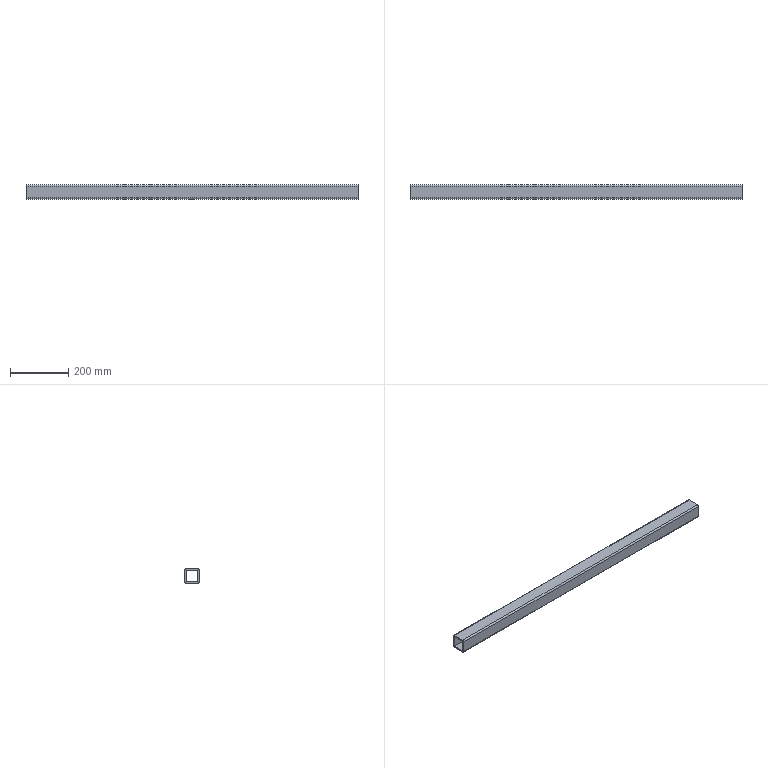Part | STEP file | SOLID | 1 solid | 15 faces | box 1140 x 50 x 50 mm | volume 1000530 mm3 | plane 10 | cylinder 5 | commonest cylinder face diameters 10 x4 16 x1
STEP:
#1=CARTESIAN_POINT('',(0.,0.,0.));
#2=DIRECTION('',(0.,0.,1.));
#3=DIRECTION('',(1.,0.,0.));
#4=AXIS2_PLACEMENT_3D('',#1,#2,#3);
#5=CARTESIAN_POINT('',(-753.5,420.,-725.));
#6=VERTEX_POINT('',#5);
#7=CARTESIAN_POINT('',(-753.5,420.,-685.));
#8=VERTEX_POINT('',#7);
#9=CARTESIAN_POINT('',(-753.5,420.,-685.));
#10=DIRECTION('',(0.,0.,1.));
#11=VECTOR('',#10,1.);
#12=LINE('',#9,#11);
#13=CARTESIAN_POINT('',(636.5,420.,-685.));
#14=DIRECTION('',(0.,-1.,0.));
#15=DIRECTION('',(0.,0.,1.));
#16=AXIS2_PLACEMENT_3D('',#13,#14,#15);
#17=PLANE('',#16);
#18=CARTESIAN_POINT('',(0.,1390.));
#19=DIRECTION('',(1.,0.));
#20=VECTOR('',#19,1.);
#21=LINE('',#18,#20);
#22=(GEOMETRIC_REPRESENTATION_CONTEXT(2)PARAMETRIC_REPRESENTATION_CONTEXT()REPRESENTATION_CONTEXT('',''));
#23=DEFINITIONAL_REPRESENTATION('',(#21),#22);
#24=PCURVE('',#17,#23);
#25=CARTESIAN_POINT('',(-753.5,380.,-670.));
#26=DIRECTION('',(-1.,0.,0.));
#27=DIRECTION('',(0.,1.,0.));
#28=AXIS2_PLACEMENT_3D('',#25,#26,#27);
#29=PLANE('',#28);
#30=CARTESIAN_POINT('',(40.,15.));
#31=DIRECTION('',(0.,-1.));
#32=VECTOR('',#31,1.);
#33=LINE('',#30,#32);
#34=(GEOMETRIC_REPRESENTATION_CONTEXT(2)PARAMETRIC_REPRESENTATION_CONTEXT()REPRESENTATION_CONTEXT('',''));
#35=DEFINITIONAL_REPRESENTATION('',(#33),#34);
#36=PCURVE('',#29,#35);
#37=SURFACE_CURVE('',#12,(#24,#36),.PCURVE_S1.);
#38=EDGE_CURVE('',#6,#8,#37,.T.);
#39=ORIENTED_EDGE('',*,*,#38,.F.);
#40=CARTESIAN_POINT('',(386.5,420.,-725.));
#41=VERTEX_POINT('',#40);
#42=CARTESIAN_POINT('',(636.5,420.,-725.));
#43=DIRECTION('',(1.,0.,0.));
#44=VECTOR('',#43,1.);
#45=LINE('',#42,#44);
#46=CARTESIAN_POINT('',(-40.,0.));
#47=DIRECTION('',(0.,-1.));
#48=VECTOR('',#47,1.);
#49=LINE('',#46,#48);
#50=(GEOMETRIC_REPRESENTATION_CONTEXT(2)PARAMETRIC_REPRESENTATION_CONTEXT()REPRESENTATION_CONTEXT('',''));
#51=DEFINITIONAL_REPRESENTATION('',(#49),#50);
#52=PCURVE('',#17,#51);
#53=CARTESIAN_POINT('',(636.5,420.,-725.));
#54=DIRECTION('',(0.,0.,1.));
#55=DIRECTION('',(0.,1.,0.));
#56=AXIS2_PLACEMENT_3D('',#53,#54,#55);
#57=PLANE('',#56);
#58=CARTESIAN_POINT('',(0.,0.));
#59=DIRECTION('',(0.,-1.));
#60=VECTOR('',#59,1.);
#61=LINE('',#58,#60);
#62=(GEOMETRIC_REPRESENTATION_CONTEXT(2)PARAMETRIC_REPRESENTATION_CONTEXT()REPRESENTATION_CONTEXT('',''));
#63=DEFINITIONAL_REPRESENTATION('',(#61),#62);
#64=PCURVE('',#57,#63);
#65=SURFACE_CURVE('',#45,(#52,#64),.PCURVE_S1.);
#66=EDGE_CURVE('',#6,#41,#65,.T.);
#67=ORIENTED_EDGE('',*,*,#66,.T.);
#68=CARTESIAN_POINT('',(386.5,420.,-685.));
#69=VERTEX_POINT('',#68);
#70=CARTESIAN_POINT('',(386.5,420.,-685.));
#71=DIRECTION('',(0.,0.,1.));
#72=VECTOR('',#71,1.);
#73=LINE('',#70,#72);
#74=CARTESIAN_POINT('',(0.,250.));
#75=DIRECTION('',(1.,0.));
#76=VECTOR('',#75,1.);
#77=LINE('',#74,#76);
#78=(GEOMETRIC_REPRESENTATION_CONTEXT(2)PARAMETRIC_REPRESENTATION_CONTEXT()REPRESENTATION_CONTEXT('',''));
#79=DEFINITIONAL_REPRESENTATION('',(#77),#78);
#80=PCURVE('',#17,#79);
#81=CARTESIAN_POINT('',(386.5,380.,-670.));
#82=DIRECTION('',(1.,0.,0.));
#83=DIRECTION('',(0.,1.,0.));
#84=AXIS2_PLACEMENT_3D('',#81,#82,#83);
#85=PLANE('',#84);
#86=CARTESIAN_POINT('',(40.,-15.));
#87=DIRECTION('',(0.,1.));
#88=VECTOR('',#87,1.);
#89=LINE('',#86,#88);
#90=(GEOMETRIC_REPRESENTATION_CONTEXT(2)PARAMETRIC_REPRESENTATION_CONTEXT()REPRESENTATION_CONTEXT('',''));
#91=DEFINITIONAL_REPRESENTATION('',(#89),#90);
#92=PCURVE('',#85,#91);
#93=SURFACE_CURVE('',#73,(#80,#92),.PCURVE_S1.);
#94=EDGE_CURVE('',#41,#69,#93,.T.);
#95=ORIENTED_EDGE('',*,*,#94,.T.);
#96=CARTESIAN_POINT('',(636.5,420.,-685.));
#97=DIRECTION('',(1.,0.,0.));
#98=VECTOR('',#97,1.);
#99=LINE('',#96,#98);
#100=CARTESIAN_POINT('',(0.,0.));
#101=DIRECTION('',(0.,-1.));
#102=VECTOR('',#101,1.);
#103=LINE('',#100,#102);
#104=(GEOMETRIC_REPRESENTATION_CONTEXT(2)PARAMETRIC_REPRESENTATION_CONTEXT()REPRESENTATION_CONTEXT('',''));
#105=DEFINITIONAL_REPRESENTATION('',(#103),#104);
#106=PCURVE('',#17,#105);
#107=CARTESIAN_POINT('',(636.5,380.,-685.));
#108=DIRECTION('',(0.,0.,-1.));
#109=DIRECTION('',(0.,-1.,0.));
#110=AXIS2_PLACEMENT_3D('',#107,#108,#109);
#111=PLANE('',#110);
#112=CARTESIAN_POINT('',(-40.,0.));
#113=DIRECTION('',(0.,-1.));
#114=VECTOR('',#113,1.);
#115=LINE('',#112,#114);
#116=(GEOMETRIC_REPRESENTATION_CONTEXT(2)PARAMETRIC_REPRESENTATION_CONTEXT()REPRESENTATION_CONTEXT('',''));
#117=DEFINITIONAL_REPRESENTATION('',(#115),#116);
#118=PCURVE('',#111,#117);
#119=SURFACE_CURVE('',#99,(#106,#118),.PCURVE_S1.);
#120=EDGE_CURVE('',#8,#69,#119,.T.);
#121=ORIENTED_EDGE('',*,*,#120,.F.);
#122=EDGE_LOOP('',(#39,#67,#95,#121));
#123=FACE_BOUND('',#122,.T.);
#124=ADVANCED_FACE('',(#123),#17,.T.);
#125=CARTESIAN_POINT('',(-753.5,380.,-685.));
#126=VERTEX_POINT('',#125);
#127=CARTESIAN_POINT('',(-753.5,380.,-685.));
#128=DIRECTION('',(0.,-1.,0.));
#129=VECTOR('',#128,1.);
#130=LINE('',#127,#129);
#131=CARTESIAN_POINT('',(0.,1390.));
#132=DIRECTION('',(1.,0.));
#133=VECTOR('',#132,1.);
#134=LINE('',#131,#133);
#135=(GEOMETRIC_REPRESENTATION_CONTEXT(2)PARAMETRIC_REPRESENTATION_CONTEXT()REPRESENTATION_CONTEXT('',''));
#136=DEFINITIONAL_REPRESENTATION('',(#134),#135);
#137=PCURVE('',#111,#136);
#138=CARTESIAN_POINT('',(0.,15.));
#139=DIRECTION('',(-1.,0.));
#140=VECTOR('',#139,1.);
#141=LINE('',#138,#140);
#142=(GEOMETRIC_REPRESENTATION_CONTEXT(2)PARAMETRIC_REPRESENTATION_CONTEXT()REPRESENTATION_CONTEXT('',''));
#143=DEFINITIONAL_REPRESENTATION('',(#141),#142);
#144=PCURVE('',#29,#143);
#145=SURFACE_CURVE('',#130,(#137,#144),.PCURVE_S1.);
#146=EDGE_CURVE('',#8,#126,#145,.T.);
#147=ORIENTED_EDGE('',*,*,#146,.F.);
#148=ORIENTED_EDGE('',*,*,#120,.T.);
#149=CARTESIAN_POINT('',(386.5,380.,-685.));
#150=VERTEX_POINT('',#149);
#151=CARTESIAN_POINT('',(386.5,380.,-685.));
#152=DIRECTION('',(0.,-1.,0.));
#153=VECTOR('',#152,1.);
#154=LINE('',#151,#153);
#155=CARTESIAN_POINT('',(0.,250.));
#156=DIRECTION('',(1.,0.));
#157=VECTOR('',#156,1.);
#158=LINE('',#155,#157);
#159=(GEOMETRIC_REPRESENTATION_CONTEXT(2)PARAMETRIC_REPRESENTATION_CONTEXT()REPRESENTATION_CONTEXT('',''));
#160=DEFINITIONAL_REPRESENTATION('',(#158),#159);
#161=PCURVE('',#111,#160);
#162=CARTESIAN_POINT('',(0.,-15.));
#163=DIRECTION('',(-1.,0.));
#164=VECTOR('',#163,1.);
#165=LINE('',#162,#164);
#166=(GEOMETRIC_REPRESENTATION_CONTEXT(2)PARAMETRIC_REPRESENTATION_CONTEXT()REPRESENTATION_CONTEXT('',''));
#167=DEFINITIONAL_REPRESENTATION('',(#165),#166);
#168=PCURVE('',#85,#167);
#169=SURFACE_CURVE('',#154,(#161,#168),.PCURVE_S1.);
#170=EDGE_CURVE('',#69,#150,#169,.T.);
#171=ORIENTED_EDGE('',*,*,#170,.T.);
#172=CARTESIAN_POINT('',(636.5,380.,-685.));
#173=DIRECTION('',(1.,0.,0.));
#174=VECTOR('',#173,1.);
#175=LINE('',#172,#174);
#176=CARTESIAN_POINT('',(0.,0.));
#177=DIRECTION('',(0.,-1.));
#178=VECTOR('',#177,1.);
#179=LINE('',#176,#178);
#180=(GEOMETRIC_REPRESENTATION_CONTEXT(2)PARAMETRIC_REPRESENTATION_CONTEXT()REPRESENTATION_CONTEXT('',''));
#181=DEFINITIONAL_REPRESENTATION('',(#179),#180);
#182=PCURVE('',#111,#181);
#183=CARTESIAN_POINT('',(636.5,380.,-725.));
#184=DIRECTION('',(0.,1.,0.));
#185=DIRECTION('',(0.,0.,-1.));
#186=AXIS2_PLACEMENT_3D('',#183,#184,#185);
#187=PLANE('',#186);
#188=CARTESIAN_POINT('',(-40.,0.));
#189=DIRECTION('',(0.,-1.));
#190=VECTOR('',#189,1.);
#191=LINE('',#188,#190);
#192=(GEOMETRIC_REPRESENTATION_CONTEXT(2)PARAMETRIC_REPRESENTATION_CONTEXT()REPRESENTATION_CONTEXT('',''));
#193=DEFINITIONAL_REPRESENTATION('',(#191),#192);
#194=PCURVE('',#187,#193);
#195=SURFACE_CURVE('',#175,(#182,#194),.PCURVE_S1.);
#196=EDGE_CURVE('',#126,#150,#195,.T.);
#197=ORIENTED_EDGE('',*,*,#196,.F.);
#198=EDGE_LOOP('',(#147,#148,#171,#197));
#199=FACE_BOUND('',#198,.T.);
#200=ADVANCED_FACE('',(#199),#111,.T.);
#201=CARTESIAN_POINT('',(-753.5,380.,-725.));
#202=VERTEX_POINT('',#201);
#203=CARTESIAN_POINT('',(-753.5,380.,-725.));
#204=DIRECTION('',(0.,0.,-1.));
#205=VECTOR('',#204,1.);
#206=LINE('',#203,#205);
#207=CARTESIAN_POINT('',(0.,1390.));
#208=DIRECTION('',(1.,0.));
#209=VECTOR('',#208,1.);
#210=LINE('',#207,#209);
#211=(GEOMETRIC_REPRESENTATION_CONTEXT(2)PARAMETRIC_REPRESENTATION_CONTEXT()REPRESENTATION_CONTEXT('',''));
#212=DEFINITIONAL_REPRESENTATION('',(#210),#211);
#213=PCURVE('',#187,#212);
#214=CARTESIAN_POINT('',(0.,55.));
#215=DIRECTION('',(0.,1.));
#216=VECTOR('',#215,1.);
#217=LINE('',#214,#216);
#218=(GEOMETRIC_REPRESENTATION_CONTEXT(2)PARAMETRIC_REPRESENTATION_CONTEXT()REPRESENTATION_CONTEXT('',''));
#219=DEFINITIONAL_REPRESENTATION('',(#217),#218);
#220=PCURVE('',#29,#219);
#221=SURFACE_CURVE('',#206,(#213,#220),.PCURVE_S1.);
#222=EDGE_CURVE('',#126,#202,#221,.T.);
#223=ORIENTED_EDGE('',*,*,#222,.F.);
#224=ORIENTED_EDGE('',*,*,#196,.T.);
#225=CARTESIAN_POINT('',(386.5,380.,-725.));
#226=VERTEX_POINT('',#225);
#227=CARTESIAN_POINT('',(386.5,380.,-725.));
#228=DIRECTION('',(0.,0.,-1.));
#229=VECTOR('',#228,1.);
#230=LINE('',#227,#229);
#231=CARTESIAN_POINT('',(0.,250.));
#232=DIRECTION('',(1.,0.));
#233=VECTOR('',#232,1.);
#234=LINE('',#231,#233);
#235=(GEOMETRIC_REPRESENTATION_CONTEXT(2)PARAMETRIC_REPRESENTATION_CONTEXT()REPRESENTATION_CONTEXT('',''));
#236=DEFINITIONAL_REPRESENTATION('',(#234),#235);
#237=PCURVE('',#187,#236);
#238=CARTESIAN_POINT('',(0.,-55.));
#239=DIRECTION('',(0.,-1.));
#240=VECTOR('',#239,1.);
#241=LINE('',#238,#240);
#242=(GEOMETRIC_REPRESENTATION_CONTEXT(2)PARAMETRIC_REPRESENTATION_CONTEXT()REPRESENTATION_CONTEXT('',''));
#243=DEFINITIONAL_REPRESENTATION('',(#241),#242);
#244=PCURVE('',#85,#243);
#245=SURFACE_CURVE('',#230,(#237,#244),.PCURVE_S1.);
#246=EDGE_CURVE('',#150,#226,#245,.T.);
#247=ORIENTED_EDGE('',*,*,#246,.T.);
#248=CARTESIAN_POINT('',(636.5,380.,-725.));
#249=DIRECTION('',(1.,0.,0.));
#250=VECTOR('',#249,1.);
#251=LINE('',#248,#250);
#252=CARTESIAN_POINT('',(0.,0.));
#253=DIRECTION('',(0.,-1.));
#254=VECTOR('',#253,1.);
#255=LINE('',#252,#254);
#256=(GEOMETRIC_REPRESENTATION_CONTEXT(2)PARAMETRIC_REPRESENTATION_CONTEXT()REPRESENTATION_CONTEXT('',''));
#257=DEFINITIONAL_REPRESENTATION('',(#255),#256);
#258=PCURVE('',#187,#257);
#259=CARTESIAN_POINT('',(-40.,0.));
#260=DIRECTION('',(0.,-1.));
#261=VECTOR('',#260,1.);
#262=LINE('',#259,#261);
#263=(GEOMETRIC_REPRESENTATION_CONTEXT(2)PARAMETRIC_REPRESENTATION_CONTEXT()REPRESENTATION_CONTEXT('',''));
#264=DEFINITIONAL_REPRESENTATION('',(#262),#263);
#265=PCURVE('',#57,#264);
#266=SURFACE_CURVE('',#251,(#258,#265),.PCURVE_S1.);
#267=EDGE_CURVE('',#202,#226,#266,.T.);
#268=ORIENTED_EDGE('',*,*,#267,.F.);
#269=EDGE_LOOP('',(#223,#224,#247,#268));
#270=FACE_BOUND('',#269,.T.);
#271=ADVANCED_FACE('',(#270),#187,.T.);
#272=CARTESIAN_POINT('',(-753.5,425.,-725.));
#273=VERTEX_POINT('',#272);
#274=CARTESIAN_POINT('',(-753.5,425.,-685.));
#275=VERTEX_POINT('',#274);
#276=CARTESIAN_POINT('',(-753.5,425.,-685.));
#277=DIRECTION('',(0.,0.,1.));
#278=VECTOR('',#277,1.);
#279=LINE('',#276,#278);
#280=CARTESIAN_POINT('',(636.5,425.,-685.));
#281=DIRECTION('',(0.,-1.,0.));
#282=DIRECTION('',(0.,0.,1.));
#283=AXIS2_PLACEMENT_3D('',#280,#281,#282);
#284=PLANE('',#283);
#285=CARTESIAN_POINT('',(0.,1390.));
#286=DIRECTION('',(1.,0.));
#287=VECTOR('',#286,1.);
#288=LINE('',#285,#287);
#289=(GEOMETRIC_REPRESENTATION_CONTEXT(2)PARAMETRIC_REPRESENTATION_CONTEXT()REPRESENTATION_CONTEXT('',''));
#290=DEFINITIONAL_REPRESENTATION('',(#288),#289);
#291=PCURVE('',#284,#290);
#292=CARTESIAN_POINT('',(45.,15.));
#293=DIRECTION('',(0.,-1.));
#294=VECTOR('',#293,1.);
#295=LINE('',#292,#294);
#296=(GEOMETRIC_REPRESENTATION_CONTEXT(2)PARAMETRIC_REPRESENTATION_CONTEXT()REPRESENTATION_CONTEXT('',''));
#297=DEFINITIONAL_REPRESENTATION('',(#295),#296);
#298=PCURVE('',#29,#297);
#299=SURFACE_CURVE('',#279,(#291,#298),.PCURVE_S1.);
#300=EDGE_CURVE('',#273,#275,#299,.T.);
#301=ORIENTED_EDGE('',*,*,#300,.T.);
#302=CARTESIAN_POINT('',(386.5,425.,-685.));
#303=VERTEX_POINT('',#302);
#304=CARTESIAN_POINT('',(636.5,425.,-685.));
#305=DIRECTION('',(1.,0.,0.));
#306=VECTOR('',#305,1.);
#307=LINE('',#304,#306);
#308=CARTESIAN_POINT('',(0.,0.));
#309=DIRECTION('',(0.,-1.));
#310=VECTOR('',#309,1.);
#311=LINE('',#308,#310);
#312=(GEOMETRIC_REPRESENTATION_CONTEXT(2)PARAMETRIC_REPRESENTATION_CONTEXT()REPRESENTATION_CONTEXT('',''));
#313=DEFINITIONAL_REPRESENTATION('',(#311),#312);
#314=PCURVE('',#284,#313);
#315=CARTESIAN_POINT('',(636.5,420.,-685.));
#316=DIRECTION('',(-1.,0.,0.));
#317=DIRECTION('',(0.,0.,1.));
#318=AXIS2_PLACEMENT_3D('',#315,#316,#317);
#319=CYLINDRICAL_SURFACE('',#318,5.);
#320=CARTESIAN_POINT('',(1.571,0.));
#321=DIRECTION('',(0.,-1.));
#322=VECTOR('',#321,1.);
#323=LINE('',#320,#322);
#324=(GEOMETRIC_REPRESENTATION_CONTEXT(2)PARAMETRIC_REPRESENTATION_CONTEXT()REPRESENTATION_CONTEXT('',''));
#325=DEFINITIONAL_REPRESENTATION('',(#323),#324);
#326=PCURVE('',#319,#325);
#327=SURFACE_CURVE('',#307,(#314,#326),.PCURVE_S1.);
#328=EDGE_CURVE('',#275,#303,#327,.T.);
#329=ORIENTED_EDGE('',*,*,#328,.T.);
#330=CARTESIAN_POINT('',(386.5,425.,-725.));
#331=VERTEX_POINT('',#330);
#332=CARTESIAN_POINT('',(386.5,425.,-685.));
#333=DIRECTION('',(0.,0.,1.));
#334=VECTOR('',#333,1.);
#335=LINE('',#332,#334);
#336=CARTESIAN_POINT('',(0.,250.));
#337=DIRECTION('',(1.,0.));
#338=VECTOR('',#337,1.);
#339=LINE('',#336,#338);
#340=(GEOMETRIC_REPRESENTATION_CONTEXT(2)PARAMETRIC_REPRESENTATION_CONTEXT()REPRESENTATION_CONTEXT('',''));
#341=DEFINITIONAL_REPRESENTATION('',(#339),#340);
#342=PCURVE('',#284,#341);
#343=CARTESIAN_POINT('',(45.,-15.));
#344=DIRECTION('',(0.,1.));
#345=VECTOR('',#344,1.);
#346=LINE('',#343,#345);
#347=(GEOMETRIC_REPRESENTATION_CONTEXT(2)PARAMETRIC_REPRESENTATION_CONTEXT()REPRESENTATION_CONTEXT('',''));
#348=DEFINITIONAL_REPRESENTATION('',(#346),#347);
#349=PCURVE('',#85,#348);
#350=SURFACE_CURVE('',#335,(#342,#349),.PCURVE_S1.);
#351=EDGE_CURVE('',#331,#303,#350,.T.);
#352=ORIENTED_EDGE('',*,*,#351,.F.);
#353=CARTESIAN_POINT('',(636.5,425.,-725.));
#354=DIRECTION('',(1.,0.,0.));
#355=VECTOR('',#354,1.);
#356=LINE('',#353,#355);
#357=CARTESIAN_POINT('',(-40.,0.));
#358=DIRECTION('',(0.,-1.));
#359=VECTOR('',#358,1.);
#360=LINE('',#357,#359);
#361=(GEOMETRIC_REPRESENTATION_CONTEXT(2)PARAMETRIC_REPRESENTATION_CONTEXT()REPRESENTATION_CONTEXT('',''));
#362=DEFINITIONAL_REPRESENTATION('',(#360),#361);
#363=PCURVE('',#284,#362);
#364=CARTESIAN_POINT('',(636.5,420.,-725.));
#365=DIRECTION('',(-1.,0.,0.));
#366=DIRECTION('',(0.,0.,1.));
#367=AXIS2_PLACEMENT_3D('',#364,#365,#366);
#368=CYLINDRICAL_SURFACE('',#367,5.);
#369=CARTESIAN_POINT('',(1.571,0.));
#370=DIRECTION('',(0.,-1.));
#371=VECTOR('',#370,1.);
#372=LINE('',#369,#371);
#373=(GEOMETRIC_REPRESENTATION_CONTEXT(2)PARAMETRIC_REPRESENTATION_CONTEXT()REPRESENTATION_CONTEXT('',''));
#374=DEFINITIONAL_REPRESENTATION('',(#372),#373);
#375=PCURVE('',#368,#374);
#376=SURFACE_CURVE('',#356,(#363,#375),.PCURVE_S1.);
#377=EDGE_CURVE('',#273,#331,#376,.T.);
#378=ORIENTED_EDGE('',*,*,#377,.F.);
#379=EDGE_LOOP('',(#301,#329,#352,#378));
#380=FACE_BOUND('',#379,.T.);
#381=ADVANCED_FACE('',(#380),#284,.F.);
#382=CARTESIAN_POINT('',(-753.5,420.,-730.));
#383=VERTEX_POINT('',#382);
#384=CARTESIAN_POINT('',(-753.5,420.,-725.));
#385=DIRECTION('',(1.,0.,0.));
#386=DIRECTION('',(0.,-1.,0.));
#387=AXIS2_PLACEMENT_3D('',#384,#385,#386);
#388=CIRCLE('',#387,5.);
#389=CARTESIAN_POINT('',(4.712,1390.));
#390=DIRECTION('',(-1.,0.));
#391=VECTOR('',#390,1.);
#392=LINE('',#389,#391);
#393=(GEOMETRIC_REPRESENTATION_CONTEXT(2)PARAMETRIC_REPRESENTATION_CONTEXT()REPRESENTATION_CONTEXT('',''));
#394=DEFINITIONAL_REPRESENTATION('',(#392),#393);
#395=PCURVE('',#368,#394);
#396=CARTESIAN_POINT('',(35.,55.));
#397=CARTESIAN_POINT('',(35.,63.66));
#398=CARTESIAN_POINT('',(42.5,59.33));
#399=CARTESIAN_POINT('',(50.,55.));
#400=CARTESIAN_POINT('',(42.5,50.67));
#401=CARTESIAN_POINT('',(35.,46.34));
#402=CARTESIAN_POINT('',(35.,55.));
#403=(BOUNDED_CURVE()B_SPLINE_CURVE(2,(#396,#397,#398,#399,#400,#401,#402),.UNSPECIFIED.,.T.,.F.)B_SPLINE_CURVE_WITH_KNOTS((1,2,2,2,2,1),(-2.094,0.,2.094,4.189,6.283,8.378),.UNSPECIFIED.)CURVE()GEOMETRIC_REPRESENTATION_ITEM()RATIONAL_B_SPLINE_CURVE((1.,0.5,1.,0.5,1.,0.5,1.))REPRESENTATION_ITEM(''));
#404=(GEOMETRIC_REPRESENTATION_CONTEXT(2)PARAMETRIC_REPRESENTATION_CONTEXT()REPRESENTATION_CONTEXT('',''));
#405=DEFINITIONAL_REPRESENTATION('',(#403),#404);
#406=PCURVE('',#29,#405);
#407=SURFACE_CURVE('',#388,(#395,#406),.PCURVE_S1.);
#408=EDGE_CURVE('',#383,#273,#407,.T.);
#409=ORIENTED_EDGE('',*,*,#408,.T.);
#410=ORIENTED_EDGE('',*,*,#377,.T.);
#411=CARTESIAN_POINT('',(386.5,420.,-730.));
#412=VERTEX_POINT('',#411);
#413=CARTESIAN_POINT('',(386.5,420.,-725.));
#414=DIRECTION('',(1.,0.,0.));
#415=DIRECTION('',(0.,1.,0.));
#416=AXIS2_PLACEMENT_3D('',#413,#414,#415);
#417=CIRCLE('',#416,5.);
#418=CARTESIAN_POINT('',(7.854,250.));
#419=DIRECTION('',(-1.,0.));
#420=VECTOR('',#419,1.);
#421=LINE('',#418,#420);
#422=(GEOMETRIC_REPRESENTATION_CONTEXT(2)PARAMETRIC_REPRESENTATION_CONTEXT()REPRESENTATION_CONTEXT('',''));
#423=DEFINITIONAL_REPRESENTATION('',(#421),#422);
#424=PCURVE('',#368,#423);
#425=CARTESIAN_POINT('',(40.,-55.));
#426=DIRECTION('',(1.,0.));
#427=AXIS2_PLACEMENT_2D('',#425,#426);
#428=CIRCLE('',#427,5.);
#429=(GEOMETRIC_REPRESENTATION_CONTEXT(2)PARAMETRIC_REPRESENTATION_CONTEXT()REPRESENTATION_CONTEXT('',''));
#430=DEFINITIONAL_REPRESENTATION('',(#428),#429);
#431=PCURVE('',#85,#430);
#432=SURFACE_CURVE('',#417,(#424,#431),.PCURVE_S1.);
#433=EDGE_CURVE('',#412,#331,#432,.T.);
#434=ORIENTED_EDGE('',*,*,#433,.F.);
#435=CARTESIAN_POINT('',(636.5,420.,-730.));
#436=DIRECTION('',(1.,0.,0.));
#437=VECTOR('',#436,1.);
#438=LINE('',#435,#437);
#439=CARTESIAN_POINT('',(3.142,0.));
#440=DIRECTION('',(0.,-1.));
#441=VECTOR('',#440,1.);
#442=LINE('',#439,#441);
#443=(GEOMETRIC_REPRESENTATION_CONTEXT(2)PARAMETRIC_REPRESENTATION_CONTEXT()REPRESENTATION_CONTEXT('',''));
#444=DEFINITIONAL_REPRESENTATION('',(#442),#443);
#445=PCURVE('',#368,#444);
#446=CARTESIAN_POINT('',(636.5,420.,-730.));
#447=DIRECTION('',(0.,0.,1.));
#448=DIRECTION('',(0.,1.,0.));
#449=AXIS2_PLACEMENT_3D('',#446,#447,#448);
#450=PLANE('',#449);
#451=CARTESIAN_POINT('',(0.,0.));
#452=DIRECTION('',(0.,-1.));
#453=VECTOR('',#452,1.);
#454=LINE('',#451,#453);
#455=(GEOMETRIC_REPRESENTATION_CONTEXT(2)PARAMETRIC_REPRESENTATION_CONTEXT()REPRESENTATION_CONTEXT('',''));
#456=DEFINITIONAL_REPRESENTATION('',(#454),#455);
#457=PCURVE('',#450,#456);
#458=SURFACE_CURVE('',#438,(#445,#457),.PCURVE_S1.);
#459=EDGE_CURVE('',#383,#412,#458,.T.);
#460=ORIENTED_EDGE('',*,*,#459,.F.);
#461=EDGE_LOOP('',(#409,#410,#434,#460));
#462=FACE_BOUND('',#461,.T.);
#463=ADVANCED_FACE('',(#462),#368,.T.);
#464=CARTESIAN_POINT('',(-183.5,392.,-730.));
#465=VERTEX_POINT('',#464);
#466=CARTESIAN_POINT('',(-183.5,400.,-730.));
#467=DIRECTION('',(0.,0.,1.));
#468=DIRECTION('',(0.,-1.,0.));
#469=AXIS2_PLACEMENT_3D('',#466,#467,#468);
#470=CIRCLE('',#469,8.);
#471=CARTESIAN_POINT('',(-20.,820.));
#472=DIRECTION('',(-1.,0.));
#473=AXIS2_PLACEMENT_2D('',#471,#472);
#474=CIRCLE('',#473,8.);
#475=(GEOMETRIC_REPRESENTATION_CONTEXT(2)PARAMETRIC_REPRESENTATION_CONTEXT()REPRESENTATION_CONTEXT('',''));
#476=DEFINITIONAL_REPRESENTATION('',(#474),#475);
#477=PCURVE('',#450,#476);
#478=CARTESIAN_POINT('',(-183.5,400.,-715.));
#479=DIRECTION('',(0.,0.,-1.));
#480=DIRECTION('',(-1.,0.,0.));
#481=AXIS2_PLACEMENT_3D('',#478,#479,#480);
#482=CYLINDRICAL_SURFACE('',#481,8.);
#483=CARTESIAN_POINT('',(10.996,15.));
#484=DIRECTION('',(-1.,0.));
#485=VECTOR('',#484,1.);
#486=LINE('',#483,#485);
#487=(GEOMETRIC_REPRESENTATION_CONTEXT(2)PARAMETRIC_REPRESENTATION_CONTEXT()REPRESENTATION_CONTEXT('',''));
#488=DEFINITIONAL_REPRESENTATION('',(#486),#487);
#489=PCURVE('',#482,#488);
#490=SURFACE_CURVE('',#470,(#477,#489),.PCURVE_S1.);
#491=EDGE_CURVE('',#465,#465,#490,.T.);
#492=ORIENTED_EDGE('',*,*,#491,.T.);
#493=EDGE_LOOP('',(#492));
#494=FACE_BOUND('',#493,.T.);
#495=CARTESIAN_POINT('',(-753.5,380.,-730.));
#496=VERTEX_POINT('',#495);
#497=CARTESIAN_POINT('',(-753.5,420.,-730.));
#498=DIRECTION('',(0.,1.,0.));
#499=VECTOR('',#498,1.);
#500=LINE('',#497,#499);
#501=CARTESIAN_POINT('',(0.,1390.));
#502=DIRECTION('',(1.,0.));
#503=VECTOR('',#502,1.);
#504=LINE('',#501,#503);
#505=(GEOMETRIC_REPRESENTATION_CONTEXT(2)PARAMETRIC_REPRESENTATION_CONTEXT()REPRESENTATION_CONTEXT('',''));
#506=DEFINITIONAL_REPRESENTATION('',(#504),#505);
#507=PCURVE('',#450,#506);
#508=CARTESIAN_POINT('',(40.,60.));
#509=DIRECTION('',(1.,0.));
#510=VECTOR('',#509,1.);
#511=LINE('',#508,#510);
#512=(GEOMETRIC_REPRESENTATION_CONTEXT(2)PARAMETRIC_REPRESENTATION_CONTEXT()REPRESENTATION_CONTEXT('',''));
#513=DEFINITIONAL_REPRESENTATION('',(#511),#512);
#514=PCURVE('',#29,#513);
#515=SURFACE_CURVE('',#500,(#507,#514),.PCURVE_S1.);
#516=EDGE_CURVE('',#496,#383,#515,.T.);
#517=ORIENTED_EDGE('',*,*,#516,.T.);
#518=ORIENTED_EDGE('',*,*,#459,.T.);
#519=CARTESIAN_POINT('',(386.5,380.,-730.));
#520=VERTEX_POINT('',#519);
#521=CARTESIAN_POINT('',(386.5,420.,-730.));
#522=DIRECTION('',(0.,1.,0.));
#523=VECTOR('',#522,1.);
#524=LINE('',#521,#523);
#525=CARTESIAN_POINT('',(0.,250.));
#526=DIRECTION('',(1.,0.));
#527=VECTOR('',#526,1.);
#528=LINE('',#525,#527);
#529=(GEOMETRIC_REPRESENTATION_CONTEXT(2)PARAMETRIC_REPRESENTATION_CONTEXT()REPRESENTATION_CONTEXT('',''));
#530=DEFINITIONAL_REPRESENTATION('',(#528),#529);
#531=PCURVE('',#450,#530);
#532=CARTESIAN_POINT('',(40.,-60.));
#533=DIRECTION('',(1.,0.));
#534=VECTOR('',#533,1.);
#535=LINE('',#532,#534);
#536=(GEOMETRIC_REPRESENTATION_CONTEXT(2)PARAMETRIC_REPRESENTATION_CONTEXT()REPRESENTATION_CONTEXT('',''));
#537=DEFINITIONAL_REPRESENTATION('',(#535),#536);
#538=PCURVE('',#85,#537);
#539=SURFACE_CURVE('',#524,(#531,#538),.PCURVE_S1.);
#540=EDGE_CURVE('',#520,#412,#539,.T.);
#541=ORIENTED_EDGE('',*,*,#540,.F.);
#542=CARTESIAN_POINT('',(636.5,380.,-730.));
#543=DIRECTION('',(1.,0.,0.));
#544=VECTOR('',#543,1.);
#545=LINE('',#542,#544);
#546=CARTESIAN_POINT('',(-40.,0.));
#547=DIRECTION('',(0.,-1.));
#548=VECTOR('',#547,1.);
#549=LINE('',#546,#548);
#550=(GEOMETRIC_REPRESENTATION_CONTEXT(2)PARAMETRIC_REPRESENTATION_CONTEXT()REPRESENTATION_CONTEXT('',''));
#551=DEFINITIONAL_REPRESENTATION('',(#549),#550);
#552=PCURVE('',#450,#551);
#553=CARTESIAN_POINT('',(636.5,380.,-725.));
#554=DIRECTION('',(-1.,0.,0.));
#555=DIRECTION('',(0.,0.,1.));
#556=AXIS2_PLACEMENT_3D('',#553,#554,#555);
#557=CYLINDRICAL_SURFACE('',#556,5.);
#558=CARTESIAN_POINT('',(3.142,0.));
#559=DIRECTION('',(0.,-1.));
#560=VECTOR('',#559,1.);
#561=LINE('',#558,#560);
#562=(GEOMETRIC_REPRESENTATION_CONTEXT(2)PARAMETRIC_REPRESENTATION_CONTEXT()REPRESENTATION_CONTEXT('',''));
#563=DEFINITIONAL_REPRESENTATION('',(#561),#562);
#564=PCURVE('',#557,#563);
#565=SURFACE_CURVE('',#545,(#552,#564),.PCURVE_S1.);
#566=EDGE_CURVE('',#496,#520,#565,.T.);
#567=ORIENTED_EDGE('',*,*,#566,.F.);
#568=EDGE_LOOP('',(#517,#518,#541,#567));
#569=FACE_BOUND('',#568,.T.);
#570=ADVANCED_FACE('',(#494,#569),#450,.F.);
#571=CARTESIAN_POINT('',(-753.5,375.,-725.));
#572=VERTEX_POINT('',#571);
#573=CARTESIAN_POINT('',(-753.5,380.,-725.));
#574=DIRECTION('',(1.,0.,0.));
#575=DIRECTION('',(0.,-1.,0.));
#576=AXIS2_PLACEMENT_3D('',#573,#574,#575);
#577=CIRCLE('',#576,5.);
#578=CARTESIAN_POINT('',(4.712,1390.));
#579=DIRECTION('',(-1.,0.));
#580=VECTOR('',#579,1.);
#581=LINE('',#578,#580);
#582=(GEOMETRIC_REPRESENTATION_CONTEXT(2)PARAMETRIC_REPRESENTATION_CONTEXT()REPRESENTATION_CONTEXT('',''));
#583=DEFINITIONAL_REPRESENTATION('',(#581),#582);
#584=PCURVE('',#557,#583);
#585=CARTESIAN_POINT('',(-5.,55.));
#586=CARTESIAN_POINT('',(-5.,63.66));
#587=CARTESIAN_POINT('',(2.5,59.33));
#588=CARTESIAN_POINT('',(10.,55.));
#589=CARTESIAN_POINT('',(2.5,50.67));
#590=CARTESIAN_POINT('',(-5.,46.34));
#591=CARTESIAN_POINT('',(-5.,55.));
#592=(BOUNDED_CURVE()B_SPLINE_CURVE(2,(#585,#586,#587,#588,#589,#590,#591),.UNSPECIFIED.,.T.,.F.)B_SPLINE_CURVE_WITH_KNOTS((1,2,2,2,2,1),(-2.094,0.,2.094,4.189,6.283,8.378),.UNSPECIFIED.)CURVE()GEOMETRIC_REPRESENTATION_ITEM()RATIONAL_B_SPLINE_CURVE((1.,0.5,1.,0.5,1.,0.5,1.))REPRESENTATION_ITEM(''));
#593=(GEOMETRIC_REPRESENTATION_CONTEXT(2)PARAMETRIC_REPRESENTATION_CONTEXT()REPRESENTATION_CONTEXT('',''));
#594=DEFINITIONAL_REPRESENTATION('',(#592),#593);
#595=PCURVE('',#29,#594);
#596=SURFACE_CURVE('',#577,(#584,#595),.PCURVE_S1.);
#597=EDGE_CURVE('',#572,#496,#596,.T.);
#598=ORIENTED_EDGE('',*,*,#597,.T.);
#599=ORIENTED_EDGE('',*,*,#566,.T.);
#600=CARTESIAN_POINT('',(386.5,375.,-725.));
#601=VERTEX_POINT('',#600);
#602=CARTESIAN_POINT('',(386.5,380.,-725.));
#603=DIRECTION('',(1.,0.,0.));
#604=DIRECTION('',(0.,1.,0.));
#605=AXIS2_PLACEMENT_3D('',#602,#603,#604);
#606=CIRCLE('',#605,5.);
#607=CARTESIAN_POINT('',(7.854,250.));
#608=DIRECTION('',(-1.,0.));
#609=VECTOR('',#608,1.);
#610=LINE('',#607,#609);
#611=(GEOMETRIC_REPRESENTATION_CONTEXT(2)PARAMETRIC_REPRESENTATION_CONTEXT()REPRESENTATION_CONTEXT('',''));
#612=DEFINITIONAL_REPRESENTATION('',(#610),#611);
#613=PCURVE('',#557,#612);
#614=CARTESIAN_POINT('',(0.,-55.));
#615=DIRECTION('',(1.,0.));
#616=AXIS2_PLACEMENT_2D('',#614,#615);
#617=CIRCLE('',#616,5.);
#618=(GEOMETRIC_REPRESENTATION_CONTEXT(2)PARAMETRIC_REPRESENTATION_CONTEXT()REPRESENTATION_CONTEXT('',''));
#619=DEFINITIONAL_REPRESENTATION('',(#617),#618);
#620=PCURVE('',#85,#619);
#621=SURFACE_CURVE('',#606,(#613,#620),.PCURVE_S1.);
#622=EDGE_CURVE('',#601,#520,#621,.T.);
#623=ORIENTED_EDGE('',*,*,#622,.F.);
#624=CARTESIAN_POINT('',(636.5,375.,-725.));
#625=DIRECTION('',(1.,0.,0.));
#626=VECTOR('',#625,1.);
#627=LINE('',#624,#626);
#628=CARTESIAN_POINT('',(4.712,0.));
#629=DIRECTION('',(0.,-1.));
#630=VECTOR('',#629,1.);
#631=LINE('',#628,#630);
#632=(GEOMETRIC_REPRESENTATION_CONTEXT(2)PARAMETRIC_REPRESENTATION_CONTEXT()REPRESENTATION_CONTEXT('',''));
#633=DEFINITIONAL_REPRESENTATION('',(#631),#632);
#634=PCURVE('',#557,#633);
#635=CARTESIAN_POINT('',(636.5,375.,-725.));
#636=DIRECTION('',(0.,1.,0.));
#637=DIRECTION('',(0.,0.,-1.));
#638=AXIS2_PLACEMENT_3D('',#635,#636,#637);
#639=PLANE('',#638);
#640=CARTESIAN_POINT('',(0.,0.));
#641=DIRECTION('',(0.,-1.));
#642=VECTOR('',#641,1.);
#643=LINE('',#640,#642);
#644=(GEOMETRIC_REPRESENTATION_CONTEXT(2)PARAMETRIC_REPRESENTATION_CONTEXT()REPRESENTATION_CONTEXT('',''));
#645=DEFINITIONAL_REPRESENTATION('',(#643),#644);
#646=PCURVE('',#639,#645);
#647=SURFACE_CURVE('',#627,(#634,#646),.PCURVE_S1.);
#648=EDGE_CURVE('',#572,#601,#647,.T.);
#649=ORIENTED_EDGE('',*,*,#648,.F.);
#650=EDGE_LOOP('',(#598,#599,#623,#649));
#651=FACE_BOUND('',#650,.T.);
#652=ADVANCED_FACE('',(#651),#557,.T.);
#653=CARTESIAN_POINT('',(-753.5,375.,-685.));
#654=VERTEX_POINT('',#653);
#655=CARTESIAN_POINT('',(-753.5,375.,-725.));
#656=DIRECTION('',(0.,0.,-1.));
#657=VECTOR('',#656,1.);
#658=LINE('',#655,#657);
#659=CARTESIAN_POINT('',(0.,1390.));
#660=DIRECTION('',(1.,0.));
#661=VECTOR('',#660,1.);
#662=LINE('',#659,#661);
#663=(GEOMETRIC_REPRESENTATION_CONTEXT(2)PARAMETRIC_REPRESENTATION_CONTEXT()REPRESENTATION_CONTEXT('',''));
#664=DEFINITIONAL_REPRESENTATION('',(#662),#663);
#665=PCURVE('',#639,#664);
#666=CARTESIAN_POINT('',(-5.,55.));
#667=DIRECTION('',(0.,1.));
#668=VECTOR('',#667,1.);
#669=LINE('',#666,#668);
#670=(GEOMETRIC_REPRESENTATION_CONTEXT(2)PARAMETRIC_REPRESENTATION_CONTEXT()REPRESENTATION_CONTEXT('',''));
#671=DEFINITIONAL_REPRESENTATION('',(#669),#670);
#672=PCURVE('',#29,#671);
#673=SURFACE_CURVE('',#658,(#665,#672),.PCURVE_S1.);
#674=EDGE_CURVE('',#654,#572,#673,.T.);
#675=ORIENTED_EDGE('',*,*,#674,.T.);
#676=ORIENTED_EDGE('',*,*,#648,.T.);
#677=CARTESIAN_POINT('',(386.5,375.,-685.));
#678=VERTEX_POINT('',#677);
#679=CARTESIAN_POINT('',(386.5,375.,-725.));
#680=DIRECTION('',(0.,0.,-1.));
#681=VECTOR('',#680,1.);
#682=LINE('',#679,#681);
#683=CARTESIAN_POINT('',(0.,250.));
#684=DIRECTION('',(1.,0.));
#685=VECTOR('',#684,1.);
#686=LINE('',#683,#685);
#687=(GEOMETRIC_REPRESENTATION_CONTEXT(2)PARAMETRIC_REPRESENTATION_CONTEXT()REPRESENTATION_CONTEXT('',''));
#688=DEFINITIONAL_REPRESENTATION('',(#686),#687);
#689=PCURVE('',#639,#688);
#690=CARTESIAN_POINT('',(-5.,-55.));
#691=DIRECTION('',(0.,-1.));
#692=VECTOR('',#691,1.);
#693=LINE('',#690,#692);
#694=(GEOMETRIC_REPRESENTATION_CONTEXT(2)PARAMETRIC_REPRESENTATION_CONTEXT()REPRESENTATION_CONTEXT('',''));
#695=DEFINITIONAL_REPRESENTATION('',(#693),#694);
#696=PCURVE('',#85,#695);
#697=SURFACE_CURVE('',#682,(#689,#696),.PCURVE_S1.);
#698=EDGE_CURVE('',#678,#601,#697,.T.);
#699=ORIENTED_EDGE('',*,*,#698,.F.);
#700=CARTESIAN_POINT('',(636.5,375.,-685.));
#701=DIRECTION('',(1.,0.,0.));
#702=VECTOR('',#701,1.);
#703=LINE('',#700,#702);
#704=CARTESIAN_POINT('',(-40.,0.));
#705=DIRECTION('',(0.,-1.));
#706=VECTOR('',#705,1.);
#707=LINE('',#704,#706);
#708=(GEOMETRIC_REPRESENTATION_CONTEXT(2)PARAMETRIC_REPRESENTATION_CONTEXT()REPRESENTATION_CONTEXT('',''));
#709=DEFINITIONAL_REPRESENTATION('',(#707),#708);
#710=PCURVE('',#639,#709);
#711=CARTESIAN_POINT('',(636.5,380.,-685.));
#712=DIRECTION('',(-1.,0.,0.));
#713=DIRECTION('',(0.,0.,1.));
#714=AXIS2_PLACEMENT_3D('',#711,#712,#713);
#715=CYLINDRICAL_SURFACE('',#714,5.);
#716=CARTESIAN_POINT('',(4.712,0.));
#717=DIRECTION('',(0.,-1.));
#718=VECTOR('',#717,1.);
#719=LINE('',#716,#718);
#720=(GEOMETRIC_REPRESENTATION_CONTEXT(2)PARAMETRIC_REPRESENTATION_CONTEXT()REPRESENTATION_CONTEXT('',''));
#721=DEFINITIONAL_REPRESENTATION('',(#719),#720);
#722=PCURVE('',#715,#721);
#723=SURFACE_CURVE('',#703,(#710,#722),.PCURVE_S1.);
#724=EDGE_CURVE('',#654,#678,#723,.T.);
#725=ORIENTED_EDGE('',*,*,#724,.F.);
#726=EDGE_LOOP('',(#675,#676,#699,#725));
#727=FACE_BOUND('',#726,.T.);
#728=ADVANCED_FACE('',(#727),#639,.F.);
#729=CARTESIAN_POINT('',(-753.5,380.,-680.));
#730=VERTEX_POINT('',#729);
#731=CARTESIAN_POINT('',(-753.5,380.,-685.));
#732=DIRECTION('',(1.,0.,0.));
#733=DIRECTION('',(0.,-1.,0.));
#734=AXIS2_PLACEMENT_3D('',#731,#732,#733);
#735=CIRCLE('',#734,5.);
#736=CARTESIAN_POINT('',(10.996,1390.));
#737=DIRECTION('',(-1.,0.));
#738=VECTOR('',#737,1.);
#739=LINE('',#736,#738);
#740=(GEOMETRIC_REPRESENTATION_CONTEXT(2)PARAMETRIC_REPRESENTATION_CONTEXT()REPRESENTATION_CONTEXT('',''));
#741=DEFINITIONAL_REPRESENTATION('',(#739),#740);
#742=PCURVE('',#715,#741);
#743=CARTESIAN_POINT('',(-5.,15.));
#744=CARTESIAN_POINT('',(-5.,23.66));
#745=CARTESIAN_POINT('',(2.5,19.33));
#746=CARTESIAN_POINT('',(10.,15.));
#747=CARTESIAN_POINT('',(2.5,10.67));
#748=CARTESIAN_POINT('',(-5.,6.34));
#749=CARTESIAN_POINT('',(-5.,15.));
#750=(BOUNDED_CURVE()B_SPLINE_CURVE(2,(#743,#744,#745,#746,#747,#748,#749),.UNSPECIFIED.,.T.,.F.)B_SPLINE_CURVE_WITH_KNOTS((1,2,2,2,2,1),(-2.094,0.,2.094,4.189,6.283,8.378),.UNSPECIFIED.)CURVE()GEOMETRIC_REPRESENTATION_ITEM()RATIONAL_B_SPLINE_CURVE((1.,0.5,1.,0.5,1.,0.5,1.))REPRESENTATION_ITEM(''));
#751=(GEOMETRIC_REPRESENTATION_CONTEXT(2)PARAMETRIC_REPRESENTATION_CONTEXT()REPRESENTATION_CONTEXT('',''));
#752=DEFINITIONAL_REPRESENTATION('',(#750),#751);
#753=PCURVE('',#29,#752);
#754=SURFACE_CURVE('',#735,(#742,#753),.PCURVE_S1.);
#755=EDGE_CURVE('',#730,#654,#754,.T.);
#756=ORIENTED_EDGE('',*,*,#755,.T.);
#757=ORIENTED_EDGE('',*,*,#724,.T.);
#758=CARTESIAN_POINT('',(386.5,380.,-680.));
#759=VERTEX_POINT('',#758);
#760=CARTESIAN_POINT('',(386.5,380.,-685.));
#761=DIRECTION('',(1.,0.,0.));
#762=DIRECTION('',(0.,1.,0.));
#763=AXIS2_PLACEMENT_3D('',#760,#761,#762);
#764=CIRCLE('',#763,5.);
#765=CARTESIAN_POINT('',(7.854,250.));
#766=DIRECTION('',(-1.,0.));
#767=VECTOR('',#766,1.);
#768=LINE('',#765,#767);
#769=(GEOMETRIC_REPRESENTATION_CONTEXT(2)PARAMETRIC_REPRESENTATION_CONTEXT()REPRESENTATION_CONTEXT('',''));
#770=DEFINITIONAL_REPRESENTATION('',(#768),#769);
#771=PCURVE('',#715,#770);
#772=CARTESIAN_POINT('',(0.,-15.));
#773=DIRECTION('',(1.,0.));
#774=AXIS2_PLACEMENT_2D('',#772,#773);
#775=CIRCLE('',#774,5.);
#776=(GEOMETRIC_REPRESENTATION_CONTEXT(2)PARAMETRIC_REPRESENTATION_CONTEXT()REPRESENTATION_CONTEXT('',''));
#777=DEFINITIONAL_REPRESENTATION('',(#775),#776);
#778=PCURVE('',#85,#777);
#779=SURFACE_CURVE('',#764,(#771,#778),.PCURVE_S1.);
#780=EDGE_CURVE('',#759,#678,#779,.T.);
#781=ORIENTED_EDGE('',*,*,#780,.F.);
#782=CARTESIAN_POINT('',(636.5,380.,-680.));
#783=DIRECTION('',(1.,0.,0.));
#784=VECTOR('',#783,1.);
#785=LINE('',#782,#784);
#786=CARTESIAN_POINT('',(6.283,0.));
#787=DIRECTION('',(0.,-1.));
#788=VECTOR('',#787,1.);
#789=LINE('',#786,#788);
#790=(GEOMETRIC_REPRESENTATION_CONTEXT(2)PARAMETRIC_REPRESENTATION_CONTEXT()REPRESENTATION_CONTEXT('',''));
#791=DEFINITIONAL_REPRESENTATION('',(#789),#790);
#792=PCURVE('',#715,#791);
#793=CARTESIAN_POINT('',(636.5,380.,-680.));
#794=DIRECTION('',(0.,0.,-1.));
#795=DIRECTION('',(0.,-1.,0.));
#796=AXIS2_PLACEMENT_3D('',#793,#794,#795);
#797=PLANE('',#796);
#798=CARTESIAN_POINT('',(0.,0.));
#799=DIRECTION('',(0.,-1.));
#800=VECTOR('',#799,1.);
#801=LINE('',#798,#800);
#802=(GEOMETRIC_REPRESENTATION_CONTEXT(2)PARAMETRIC_REPRESENTATION_CONTEXT()REPRESENTATION_CONTEXT('',''));
#803=DEFINITIONAL_REPRESENTATION('',(#801),#802);
#804=PCURVE('',#797,#803);
#805=SURFACE_CURVE('',#785,(#792,#804),.PCURVE_S1.);
#806=EDGE_CURVE('',#730,#759,#805,.T.);
#807=ORIENTED_EDGE('',*,*,#806,.F.);
#808=EDGE_LOOP('',(#756,#757,#781,#807));
#809=FACE_BOUND('',#808,.T.);
#810=ADVANCED_FACE('',(#809),#715,.T.);
#811=CARTESIAN_POINT('',(-753.5,420.,-680.));
#812=VERTEX_POINT('',#811);
#813=CARTESIAN_POINT('',(-753.5,380.,-680.));
#814=DIRECTION('',(0.,-1.,0.));
#815=VECTOR('',#814,1.);
#816=LINE('',#813,#815);
#817=CARTESIAN_POINT('',(0.,1390.));
#818=DIRECTION('',(1.,0.));
#819=VECTOR('',#818,1.);
#820=LINE('',#817,#819);
#821=(GEOMETRIC_REPRESENTATION_CONTEXT(2)PARAMETRIC_REPRESENTATION_CONTEXT()REPRESENTATION_CONTEXT('',''));
#822=DEFINITIONAL_REPRESENTATION('',(#820),#821);
#823=PCURVE('',#797,#822);
#824=CARTESIAN_POINT('',(0.,10.));
#825=DIRECTION('',(-1.,0.));
#826=VECTOR('',#825,1.);
#827=LINE('',#824,#826);
#828=(GEOMETRIC_REPRESENTATION_CONTEXT(2)PARAMETRIC_REPRESENTATION_CONTEXT()REPRESENTATION_CONTEXT('',''));
#829=DEFINITIONAL_REPRESENTATION('',(#827),#828);
#830=PCURVE('',#29,#829);
#831=SURFACE_CURVE('',#816,(#823,#830),.PCURVE_S1.);
#832=EDGE_CURVE('',#812,#730,#831,.T.);
#833=ORIENTED_EDGE('',*,*,#832,.T.);
#834=ORIENTED_EDGE('',*,*,#806,.T.);
#835=CARTESIAN_POINT('',(386.5,420.,-680.));
#836=VERTEX_POINT('',#835);
#837=CARTESIAN_POINT('',(386.5,380.,-680.));
#838=DIRECTION('',(0.,-1.,0.));
#839=VECTOR('',#838,1.);
#840=LINE('',#837,#839);
#841=CARTESIAN_POINT('',(0.,250.));
#842=DIRECTION('',(1.,0.));
#843=VECTOR('',#842,1.);
#844=LINE('',#841,#843);
#845=(GEOMETRIC_REPRESENTATION_CONTEXT(2)PARAMETRIC_REPRESENTATION_CONTEXT()REPRESENTATION_CONTEXT('',''));
#846=DEFINITIONAL_REPRESENTATION('',(#844),#845);
#847=PCURVE('',#797,#846);
#848=CARTESIAN_POINT('',(0.,-10.));
#849=DIRECTION('',(-1.,0.));
#850=VECTOR('',#849,1.);
#851=LINE('',#848,#850);
#852=(GEOMETRIC_REPRESENTATION_CONTEXT(2)PARAMETRIC_REPRESENTATION_CONTEXT()REPRESENTATION_CONTEXT('',''));
#853=DEFINITIONAL_REPRESENTATION('',(#851),#852);
#854=PCURVE('',#85,#853);
#855=SURFACE_CURVE('',#840,(#847,#854),.PCURVE_S1.);
#856=EDGE_CURVE('',#836,#759,#855,.T.);
#857=ORIENTED_EDGE('',*,*,#856,.F.);
#858=CARTESIAN_POINT('',(636.5,420.,-680.));
#859=DIRECTION('',(1.,0.,0.));
#860=VECTOR('',#859,1.);
#861=LINE('',#858,#860);
#862=CARTESIAN_POINT('',(-40.,0.));
#863=DIRECTION('',(0.,-1.));
#864=VECTOR('',#863,1.);
#865=LINE('',#862,#864);
#866=(GEOMETRIC_REPRESENTATION_CONTEXT(2)PARAMETRIC_REPRESENTATION_CONTEXT()REPRESENTATION_CONTEXT('',''));
#867=DEFINITIONAL_REPRESENTATION('',(#865),#866);
#868=PCURVE('',#797,#867);
#869=CARTESIAN_POINT('',(0.,0.));
#870=DIRECTION('',(0.,-1.));
#871=VECTOR('',#870,1.);
#872=LINE('',#869,#871);
#873=(GEOMETRIC_REPRESENTATION_CONTEXT(2)PARAMETRIC_REPRESENTATION_CONTEXT()REPRESENTATION_CONTEXT('',''));
#874=DEFINITIONAL_REPRESENTATION('',(#872),#873);
#875=PCURVE('',#319,#874);
#876=SURFACE_CURVE('',#861,(#868,#875),.PCURVE_S1.);
#877=EDGE_CURVE('',#812,#836,#876,.T.);
#878=ORIENTED_EDGE('',*,*,#877,.F.);
#879=EDGE_LOOP('',(#833,#834,#857,#878));
#880=FACE_BOUND('',#879,.T.);
#881=ADVANCED_FACE('',(#880),#797,.F.);
#882=CARTESIAN_POINT('',(-753.5,420.,-685.));
#883=DIRECTION('',(1.,0.,0.));
#884=DIRECTION('',(0.,-1.,0.));
#885=AXIS2_PLACEMENT_3D('',#882,#883,#884);
#886=CIRCLE('',#885,5.);
#887=CARTESIAN_POINT('',(4.712,1390.));
#888=DIRECTION('',(-1.,0.));
#889=VECTOR('',#888,1.);
#890=LINE('',#887,#889);
#891=(GEOMETRIC_REPRESENTATION_CONTEXT(2)PARAMETRIC_REPRESENTATION_CONTEXT()REPRESENTATION_CONTEXT('',''));
#892=DEFINITIONAL_REPRESENTATION('',(#890),#891);
#893=PCURVE('',#319,#892);
#894=CARTESIAN_POINT('',(35.,15.));
#895=CARTESIAN_POINT('',(35.,23.66));
#896=CARTESIAN_POINT('',(42.5,19.33));
#897=CARTESIAN_POINT('',(50.,15.));
#898=CARTESIAN_POINT('',(42.5,10.67));
#899=CARTESIAN_POINT('',(35.,6.34));
#900=CARTESIAN_POINT('',(35.,15.));
#901=(BOUNDED_CURVE()B_SPLINE_CURVE(2,(#894,#895,#896,#897,#898,#899,#900),.UNSPECIFIED.,.T.,.F.)B_SPLINE_CURVE_WITH_KNOTS((1,2,2,2,2,1),(-2.094,0.,2.094,4.189,6.283,8.378),.UNSPECIFIED.)CURVE()GEOMETRIC_REPRESENTATION_ITEM()RATIONAL_B_SPLINE_CURVE((1.,0.5,1.,0.5,1.,0.5,1.))REPRESENTATION_ITEM(''));
#902=(GEOMETRIC_REPRESENTATION_CONTEXT(2)PARAMETRIC_REPRESENTATION_CONTEXT()REPRESENTATION_CONTEXT('',''));
#903=DEFINITIONAL_REPRESENTATION('',(#901),#902);
#904=PCURVE('',#29,#903);
#905=SURFACE_CURVE('',#886,(#893,#904),.PCURVE_S1.);
#906=EDGE_CURVE('',#275,#812,#905,.T.);
#907=ORIENTED_EDGE('',*,*,#906,.T.);
#908=ORIENTED_EDGE('',*,*,#877,.T.);
#909=CARTESIAN_POINT('',(386.5,420.,-685.));
#910=DIRECTION('',(1.,0.,0.));
#911=DIRECTION('',(0.,1.,0.));
#912=AXIS2_PLACEMENT_3D('',#909,#910,#911);
#913=CIRCLE('',#912,5.);
#914=CARTESIAN_POINT('',(1.571,250.));
#915=DIRECTION('',(-1.,0.));
#916=VECTOR('',#915,1.);
#917=LINE('',#914,#916);
#918=(GEOMETRIC_REPRESENTATION_CONTEXT(2)PARAMETRIC_REPRESENTATION_CONTEXT()REPRESENTATION_CONTEXT('',''));
#919=DEFINITIONAL_REPRESENTATION('',(#917),#918);
#920=PCURVE('',#319,#919);
#921=CARTESIAN_POINT('',(40.,-15.));
#922=DIRECTION('',(1.,0.));
#923=AXIS2_PLACEMENT_2D('',#921,#922);
#924=CIRCLE('',#923,5.);
#925=(GEOMETRIC_REPRESENTATION_CONTEXT(2)PARAMETRIC_REPRESENTATION_CONTEXT()REPRESENTATION_CONTEXT('',''));
#926=DEFINITIONAL_REPRESENTATION('',(#924),#925);
#927=PCURVE('',#85,#926);
#928=SURFACE_CURVE('',#913,(#920,#927),.PCURVE_S1.);
#929=EDGE_CURVE('',#303,#836,#928,.T.);
#930=ORIENTED_EDGE('',*,*,#929,.F.);
#931=ORIENTED_EDGE('',*,*,#328,.F.);
#932=EDGE_LOOP('',(#907,#908,#930,#931));
#933=FACE_BOUND('',#932,.T.);
#934=ADVANCED_FACE('',(#933),#319,.T.);
#935=CARTESIAN_POINT('',(-183.5,392.,-725.));
#936=VERTEX_POINT('',#935);
#937=CARTESIAN_POINT('',(-183.5,400.,-725.));
#938=DIRECTION('',(0.,0.,1.));
#939=DIRECTION('',(0.,-1.,0.));
#940=AXIS2_PLACEMENT_3D('',#937,#938,#939);
#941=CIRCLE('',#940,8.);
#942=CARTESIAN_POINT('',(-20.,820.));
#943=DIRECTION('',(-1.,0.));
#944=AXIS2_PLACEMENT_2D('',#942,#943);
#945=CIRCLE('',#944,8.);
#946=(GEOMETRIC_REPRESENTATION_CONTEXT(2)PARAMETRIC_REPRESENTATION_CONTEXT()REPRESENTATION_CONTEXT('',''));
#947=DEFINITIONAL_REPRESENTATION('',(#945),#946);
#948=PCURVE('',#57,#947);
#949=CARTESIAN_POINT('',(10.996,10.));
#950=DIRECTION('',(-1.,0.));
#951=VECTOR('',#950,1.);
#952=LINE('',#949,#951);
#953=(GEOMETRIC_REPRESENTATION_CONTEXT(2)PARAMETRIC_REPRESENTATION_CONTEXT()REPRESENTATION_CONTEXT('',''));
#954=DEFINITIONAL_REPRESENTATION('',(#952),#953);
#955=PCURVE('',#482,#954);
#956=SURFACE_CURVE('',#941,(#948,#955),.PCURVE_S1.);
#957=EDGE_CURVE('',#936,#936,#956,.T.);
#958=ORIENTED_EDGE('',*,*,#957,.F.);
#959=EDGE_LOOP('',(#958));
#960=FACE_BOUND('',#959,.T.);
#961=CARTESIAN_POINT('',(-753.5,420.,-725.));
#962=DIRECTION('',(0.,1.,0.));
#963=VECTOR('',#962,1.);
#964=LINE('',#961,#963);
#965=CARTESIAN_POINT('',(0.,1390.));
#966=DIRECTION('',(1.,0.));
#967=VECTOR('',#966,1.);
#968=LINE('',#965,#967);
#969=(GEOMETRIC_REPRESENTATION_CONTEXT(2)PARAMETRIC_REPRESENTATION_CONTEXT()REPRESENTATION_CONTEXT('',''));
#970=DEFINITIONAL_REPRESENTATION('',(#968),#969);
#971=PCURVE('',#57,#970);
#972=CARTESIAN_POINT('',(40.,55.));
#973=DIRECTION('',(1.,0.));
#974=VECTOR('',#973,1.);
#975=LINE('',#972,#974);
#976=(GEOMETRIC_REPRESENTATION_CONTEXT(2)PARAMETRIC_REPRESENTATION_CONTEXT()REPRESENTATION_CONTEXT('',''));
#977=DEFINITIONAL_REPRESENTATION('',(#975),#976);
#978=PCURVE('',#29,#977);
#979=SURFACE_CURVE('',#964,(#971,#978),.PCURVE_S1.);
#980=EDGE_CURVE('',#202,#6,#979,.T.);
#981=ORIENTED_EDGE('',*,*,#980,.F.);
#982=ORIENTED_EDGE('',*,*,#267,.T.);
#983=CARTESIAN_POINT('',(386.5,420.,-725.));
#984=DIRECTION('',(0.,1.,0.));
#985=VECTOR('',#984,1.);
#986=LINE('',#983,#985);
#987=CARTESIAN_POINT('',(0.,250.));
#988=DIRECTION('',(1.,0.));
#989=VECTOR('',#988,1.);
#990=LINE('',#987,#989);
#991=(GEOMETRIC_REPRESENTATION_CONTEXT(2)PARAMETRIC_REPRESENTATION_CONTEXT()REPRESENTATION_CONTEXT('',''));
#992=DEFINITIONAL_REPRESENTATION('',(#990),#991);
#993=PCURVE('',#57,#992);
#994=CARTESIAN_POINT('',(40.,-55.));
#995=DIRECTION('',(1.,0.));
#996=VECTOR('',#995,1.);
#997=LINE('',#994,#996);
#998=(GEOMETRIC_REPRESENTATION_CONTEXT(2)PARAMETRIC_REPRESENTATION_CONTEXT()REPRESENTATION_CONTEXT('',''));
#999=DEFINITIONAL_REPRESENTATION('',(#997),#998);
#1000=PCURVE('',#85,#999);
#1001=SURFACE_CURVE('',#986,(#993,#1000),.PCURVE_S1.);
#1002=EDGE_CURVE('',#226,#41,#1001,.T.);
#1003=ORIENTED_EDGE('',*,*,#1002,.T.);
#1004=ORIENTED_EDGE('',*,*,#66,.F.);
#1005=EDGE_LOOP('',(#981,#982,#1003,#1004));
#1006=FACE_BOUND('',#1005,.T.);
#1007=ADVANCED_FACE('',(#960,#1006),#57,.T.);
#1008=ORIENTED_EDGE('',*,*,#351,.T.);
#1009=ORIENTED_EDGE('',*,*,#929,.T.);
#1010=ORIENTED_EDGE('',*,*,#856,.T.);
#1011=ORIENTED_EDGE('',*,*,#780,.T.);
#1012=ORIENTED_EDGE('',*,*,#698,.T.);
#1013=ORIENTED_EDGE('',*,*,#622,.T.);
#1014=ORIENTED_EDGE('',*,*,#540,.T.);
#1015=ORIENTED_EDGE('',*,*,#433,.T.);
#1016=EDGE_LOOP('',(#1008,#1009,#1010,#1011,#1012,#1013,#1014,#1015));
#1017=FACE_BOUND('',#1016,.T.);
#1018=ORIENTED_EDGE('',*,*,#94,.F.);
#1019=ORIENTED_EDGE('',*,*,#1002,.F.);
#1020=ORIENTED_EDGE('',*,*,#246,.F.);
#1021=ORIENTED_EDGE('',*,*,#170,.F.);
#1022=EDGE_LOOP('',(#1018,#1019,#1020,#1021));
#1023=FACE_BOUND('',#1022,.T.);
#1024=ADVANCED_FACE('',(#1017,#1023),#85,.T.);
#1025=ORIENTED_EDGE('',*,*,#300,.F.);
#1026=ORIENTED_EDGE('',*,*,#408,.F.);
#1027=ORIENTED_EDGE('',*,*,#516,.F.);
#1028=ORIENTED_EDGE('',*,*,#597,.F.);
#1029=ORIENTED_EDGE('',*,*,#674,.F.);
#1030=ORIENTED_EDGE('',*,*,#755,.F.);
#1031=ORIENTED_EDGE('',*,*,#832,.F.);
#1032=ORIENTED_EDGE('',*,*,#906,.F.);
#1033=EDGE_LOOP('',(#1025,#1026,#1027,#1028,#1029,#1030,#1031,#1032));
#1034=FACE_BOUND('',#1033,.T.);
#1035=ORIENTED_EDGE('',*,*,#38,.T.);
#1036=ORIENTED_EDGE('',*,*,#146,.T.);
#1037=ORIENTED_EDGE('',*,*,#222,.T.);
#1038=ORIENTED_EDGE('',*,*,#980,.T.);
#1039=EDGE_LOOP('',(#1035,#1036,#1037,#1038));
#1040=FACE_BOUND('',#1039,.T.);
#1041=ADVANCED_FACE('',(#1034,#1040),#29,.T.);
#1042=ORIENTED_EDGE('',*,*,#957,.F.);
#1043=CARTESIAN_POINT('',(-183.5,392.,-725.));
#1044=CARTESIAN_POINT('',(-183.5,392.,-730.));
#1045=B_SPLINE_CURVE_WITH_KNOTS('',1,(#1043,#1044),.UNSPECIFIED.,.F.,.F.,(2,2),(10.,15.),.PIECEWISE_BEZIER_KNOTS.);
#1046=CARTESIAN_POINT('',(10.996,0.));
#1047=DIRECTION('',(0.,1.));
#1048=VECTOR('',#1047,1.);
#1049=LINE('',#1046,#1048);
#1050=(GEOMETRIC_REPRESENTATION_CONTEXT(2)PARAMETRIC_REPRESENTATION_CONTEXT()REPRESENTATION_CONTEXT('',''));
#1051=DEFINITIONAL_REPRESENTATION('',(#1049),#1050);
#1052=PCURVE('',#482,#1051);
#1053=CARTESIAN_POINT('',(4.712,0.));
#1054=DIRECTION('',(0.,1.));
#1055=VECTOR('',#1054,1.);
#1056=LINE('',#1053,#1055);
#1057=(GEOMETRIC_REPRESENTATION_CONTEXT(2)PARAMETRIC_REPRESENTATION_CONTEXT()REPRESENTATION_CONTEXT('',''));
#1058=DEFINITIONAL_REPRESENTATION('',(#1056),#1057);
#1059=PCURVE('',#482,#1058);
#1060=SEAM_CURVE('',#1045,(#1052,#1059),.PCURVE_S1.);
#1061=EDGE_CURVE('',#936,#465,#1060,.T.);
#1062=ORIENTED_EDGE('',*,*,#1061,.T.);
#1063=ORIENTED_EDGE('',*,*,#491,.T.);
#1064=ORIENTED_EDGE('',*,*,#1061,.F.);
#1065=EDGE_LOOP('',(#1042,#1062,#1063,#1064));
#1066=FACE_BOUND('',#1065,.F.);
#1067=ADVANCED_FACE('',(#1066),#482,.F.);
#1068=CLOSED_SHELL('',(#124,#200,#271,#381,#463,#570,#652,#728,#810,#881,#934,#1007,#1024,#1041,#1067));
#1069=MANIFOLD_SOLID_BREP('',#1068);
#1070=(LENGTH_UNIT()NAMED_UNIT(*)SI_UNIT(.MILLI.,.METRE.));
#1071=UNCERTAINTY_MEASURE_WITH_UNIT(LENGTH_MEASURE(0.0000005),#1070,'','');
#1072=(NAMED_UNIT(*)PLANE_ANGLE_UNIT()SI_UNIT($,.RADIAN.));
#1073=(NAMED_UNIT(*)SI_UNIT($,.STERADIAN.)SOLID_ANGLE_UNIT());
#1074=(GEOMETRIC_REPRESENTATION_CONTEXT(3)GLOBAL_UNCERTAINTY_ASSIGNED_CONTEXT((#1071))GLOBAL_UNIT_ASSIGNED_CONTEXT((#1070,#1072,#1073))REPRESENTATION_CONTEXT('',''));
#1075=ADVANCED_BREP_SHAPE_REPRESENTATION('',(#4,#1069),#1074);